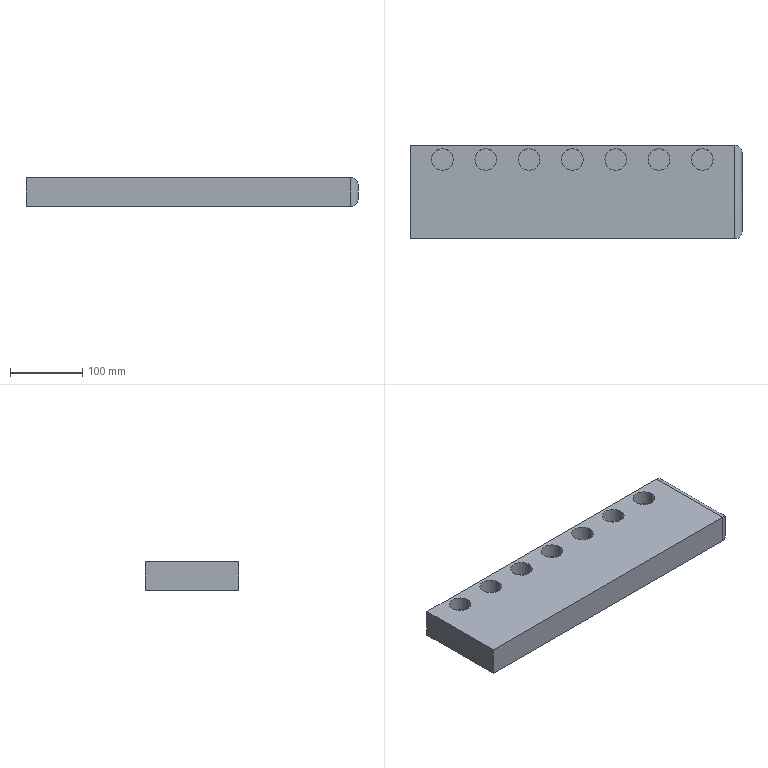Part | STEP file | 1 solid | 31 faces | box 460 x 130 x 40 mm | volume 2286127 mm3 | cylinder 18 | plane 13 | commonest cylinder face diameters 30 x14 20 x4